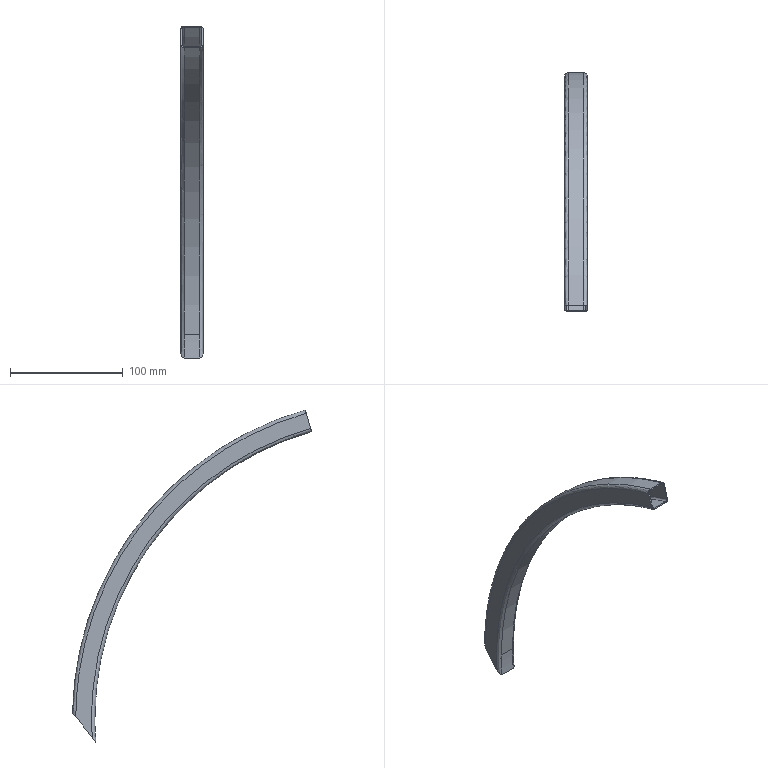Part | SolidWorks | features BaseBody 1 | 1 solid | 20 faces | box 20 x 212.461 x 295.029 mm | volume 30994 mm3 | spline 8 | cylinder 6 | plane 6 | commonest cylinder face diameters 530 x2 532.4 x2 567.6 x1 570 x1